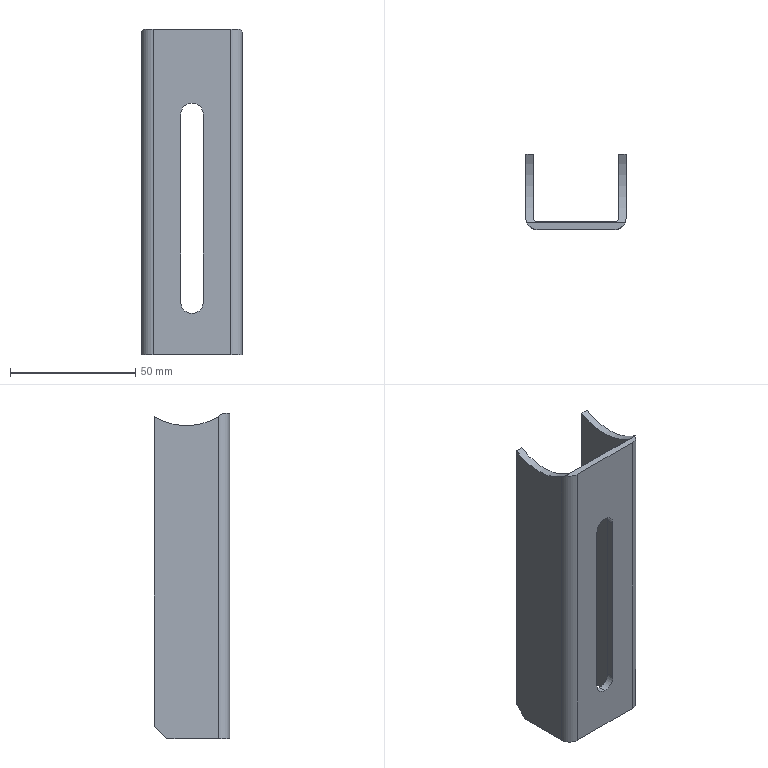Part | SolidWorks | features ICE 2, Chamfer 1, Extrusion 1 | 1 solid | 22 faces | box 40 x 30 x 130 mm | volume 32768 mm3 | plane 14 | cylinder 8 | commonest cylinder face diameters 9 x5 3 x2 48.3 x1
STEP:
#1=CARTESIAN_POINT('',(20.,-27.,16.5));
#2=VERTEX_POINT('',#1);
#3=CARTESIAN_POINT('',(24.5,-27.,21.));
#4=VERTEX_POINT('',#3);
#5=CARTESIAN_POINT('',(20.,-27.,21.));
#6=DIRECTION('',(0.,-1.,0.));
#7=DIRECTION('',(1.,0.,0.));
#8=AXIS2_PLACEMENT_3D('',#5,#6,#7);
#9=CIRCLE('',#8,4.5);
#10=EDGE_CURVE('',#2,#4,#9,.T.);
#11=ORIENTED_EDGE('',*,*,#10,.F.);
#12=CARTESIAN_POINT('',(20.,-30.,16.5));
#13=VERTEX_POINT('',#12);
#14=CARTESIAN_POINT('',(20.,100.,16.5));
#15=DIRECTION('',(0.,-1.,0.));
#16=VECTOR('',#15,1000.);
#17=LINE('',#14,#16);
#18=EDGE_CURVE('',#2,#13,#17,.T.);
#19=ORIENTED_EDGE('',*,*,#18,.T.);
#20=CARTESIAN_POINT('',(24.5,-30.,21.));
#21=VERTEX_POINT('',#20);
#22=CARTESIAN_POINT('',(20.,-30.,21.));
#23=DIRECTION('',(0.,-1.,0.));
#24=DIRECTION('',(0.,0.,-1.));
#25=AXIS2_PLACEMENT_3D('',#22,#23,#24);
#26=CIRCLE('',#25,4.5);
#27=EDGE_CURVE('',#13,#21,#26,.T.);
#28=ORIENTED_EDGE('',*,*,#27,.T.);
#29=CARTESIAN_POINT('',(24.5,100.,21.));
#30=DIRECTION('',(0.,-1.,0.));
#31=VECTOR('',#30,1000.);
#32=LINE('',#29,#31);
#33=EDGE_CURVE('',#4,#21,#32,.T.);
#34=ORIENTED_EDGE('',*,*,#33,.F.);
#35=EDGE_LOOP('',(#11,#19,#28,#34));
#36=FACE_OUTER_BOUND('',#35,.T.);
#37=CARTESIAN_POINT('',(20.,100.,21.));
#38=DIRECTION('',(0.,-1.,0.));
#39=DIRECTION('',(0.,0.,-1.));
#40=AXIS2_PLACEMENT_3D('',#37,#38,#39);
#41=CYLINDRICAL_SURFACE('',#40,4.5);
#42=ADVANCED_FACE('',(#36),#41,.F.);
#43=CARTESIAN_POINT('',(0.,0.,128.64));
#44=VERTEX_POINT('',#43);
#45=CARTESIAN_POINT('',(0.,0.,5.));
#46=VERTEX_POINT('',#45);
#47=CARTESIAN_POINT('',(0.,0.,130.));
#48=DIRECTION('',(0.,0.,-1.));
#49=VECTOR('',#48,1000.);
#50=LINE('',#47,#49);
#51=EDGE_CURVE('',#44,#46,#50,.T.);
#52=ORIENTED_EDGE('',*,*,#51,.F.);
#53=CARTESIAN_POINT('',(3.,0.,128.64));
#54=VERTEX_POINT('',#53);
#55=CARTESIAN_POINT('',(-90.,0.,128.64));
#56=DIRECTION('',(1.,0.,0.));
#57=VECTOR('',#56,1000.);
#58=LINE('',#55,#57);
#59=EDGE_CURVE('',#44,#54,#58,.T.);
#60=ORIENTED_EDGE('',*,*,#59,.T.);
#61=CARTESIAN_POINT('',(3.,0.,5.));
#62=VERTEX_POINT('',#61);
#63=CARTESIAN_POINT('',(3.,0.,130.));
#64=DIRECTION('',(0.,0.,-1.));
#65=VECTOR('',#64,1000.);
#66=LINE('',#63,#65);
#67=EDGE_CURVE('',#54,#62,#66,.T.);
#68=ORIENTED_EDGE('',*,*,#67,.T.);
#69=CARTESIAN_POINT('',(3.,0.,5.));
#70=DIRECTION('',(-1.,0.,0.));
#71=VECTOR('',#70,1000.);
#72=LINE('',#69,#71);
#73=EDGE_CURVE('',#62,#46,#72,.T.);
#74=ORIENTED_EDGE('',*,*,#73,.T.);
#75=EDGE_LOOP('',(#52,#60,#68,#74));
#76=FACE_OUTER_BOUND('',#75,.T.);
#77=CARTESIAN_POINT('',(3.,0.,130.));
#78=DIRECTION('',(0.,-1.,0.));
#79=DIRECTION('',(0.,0.,-1.));
#80=AXIS2_PLACEMENT_3D('',#77,#78,#79);
#81=PLANE('',#80);
#82=ADVANCED_FACE('',(#76),#81,.F.);
#83=CARTESIAN_POINT('',(0.,-25.5,128.64));
#84=VERTEX_POINT('',#83);
#85=CARTESIAN_POINT('',(0.,-25.5,0.));
#86=VERTEX_POINT('',#85);
#87=CARTESIAN_POINT('',(0.,-25.5,130.));
#88=DIRECTION('',(0.,0.,-1.));
#89=VECTOR('',#88,1000.);
#90=LINE('',#87,#89);
#91=EDGE_CURVE('',#84,#86,#90,.T.);
#92=ORIENTED_EDGE('',*,*,#91,.F.);
#93=CARTESIAN_POINT('',(0.,-12.75,149.15));
#94=DIRECTION('',(1.,0.,0.));
#95=DIRECTION('',(0.,1.,0.));
#96=AXIS2_PLACEMENT_3D('',#93,#94,#95);
#97=CIRCLE('',#96,24.15);
#98=EDGE_CURVE('',#84,#44,#97,.T.);
#99=ORIENTED_EDGE('',*,*,#98,.T.);
#100=ORIENTED_EDGE('',*,*,#51,.T.);
#101=CARTESIAN_POINT('',(0.,-5.,0.));
#102=VERTEX_POINT('',#101);
#103=CARTESIAN_POINT('',(0.,0.,5.));
#104=DIRECTION('',(0.,-0.7071,-0.7071));
#105=VECTOR('',#104,1000.);
#106=LINE('',#103,#105);
#107=EDGE_CURVE('',#46,#102,#106,.T.);
#108=ORIENTED_EDGE('',*,*,#107,.T.);
#109=CARTESIAN_POINT('',(0.,0.,0.));
#110=DIRECTION('',(0.,-1.,0.));
#111=VECTOR('',#110,1000.);
#112=LINE('',#109,#111);
#113=EDGE_CURVE('',#102,#86,#112,.T.);
#114=ORIENTED_EDGE('',*,*,#113,.T.);
#115=EDGE_LOOP('',(#92,#99,#100,#108,#114));
#116=FACE_OUTER_BOUND('',#115,.T.);
#117=CARTESIAN_POINT('',(0.,0.,130.));
#118=DIRECTION('',(1.,0.,0.));
#119=DIRECTION('',(0.,1.,0.));
#120=AXIS2_PLACEMENT_3D('',#117,#118,#119);
#121=PLANE('',#120);
#122=ADVANCED_FACE('',(#116),#121,.F.);
#123=CARTESIAN_POINT('',(0.4512,-27.464,130.));
#124=VERTEX_POINT('',#123);
#125=CARTESIAN_POINT('',(4.5,-30.,130.));
#126=VERTEX_POINT('',#125);
#127=CARTESIAN_POINT('',(4.5,-25.5,130.));
#128=DIRECTION('',(0.,0.,1.));
#129=DIRECTION('',(1.,0.,0.));
#130=AXIS2_PLACEMENT_3D('',#127,#128,#129);
#131=CIRCLE('',#130,4.5);
#132=EDGE_CURVE('',#124,#126,#131,.T.);
#133=ORIENTED_EDGE('',*,*,#132,.F.);
#134=CARTESIAN_POINT('',(0.4512,-27.464,130.));
#135=CARTESIAN_POINT('',(0.3031,-27.159,129.766));
#136=CARTESIAN_POINT('',(0.1919,-26.843,129.534));
#137=CARTESIAN_POINT('',(0.04037,-26.189,129.081));
#138=CARTESIAN_POINT('',(0.,-25.851,128.858));
#139=CARTESIAN_POINT('',(0.,-25.5,128.64));
#140=B_SPLINE_CURVE_WITH_KNOTS('',3,(#134,#135,#136,#137,#138,#139),.UNSPECIFIED.,.F.,.F.,(4,2,4),(0.,0.001216,0.002431),.UNSPECIFIED.);
#141=EDGE_CURVE('',#124,#84,#140,.T.);
#142=ORIENTED_EDGE('',*,*,#141,.T.);
#143=ORIENTED_EDGE('',*,*,#91,.T.);
#144=CARTESIAN_POINT('',(4.5,-30.,0.));
#145=VERTEX_POINT('',#144);
#146=CARTESIAN_POINT('',(4.5,-25.5,0.));
#147=DIRECTION('',(0.,0.,1.));
#148=DIRECTION('',(1.,0.,0.));
#149=AXIS2_PLACEMENT_3D('',#146,#147,#148);
#150=CIRCLE('',#149,4.5);
#151=EDGE_CURVE('',#86,#145,#150,.T.);
#152=ORIENTED_EDGE('',*,*,#151,.T.);
#153=CARTESIAN_POINT('',(4.5,-30.,130.));
#154=DIRECTION('',(0.,0.,-1.));
#155=VECTOR('',#154,1000.);
#156=LINE('',#153,#155);
#157=EDGE_CURVE('',#126,#145,#156,.T.);
#158=ORIENTED_EDGE('',*,*,#157,.F.);
#159=EDGE_LOOP('',(#133,#142,#143,#152,#158));
#160=FACE_OUTER_BOUND('',#159,.T.);
#161=CARTESIAN_POINT('',(4.5,-25.5,130.));
#162=DIRECTION('',(0.,0.,-1.));
#163=DIRECTION('',(-1.,0.,0.));
#164=AXIS2_PLACEMENT_3D('',#161,#162,#163);
#165=CYLINDRICAL_SURFACE('',#164,4.5);
#166=ADVANCED_FACE('',(#160),#165,.T.);
#167=CARTESIAN_POINT('',(15.5,-30.,96.));
#168=VERTEX_POINT('',#167);
#169=CARTESIAN_POINT('',(15.5,-30.,21.));
#170=VERTEX_POINT('',#169);
#171=CARTESIAN_POINT('',(15.5,-30.,96.));
#172=DIRECTION('',(0.,0.,-1.));
#173=VECTOR('',#172,1000.);
#174=LINE('',#171,#173);
#175=EDGE_CURVE('',#168,#170,#174,.T.);
#176=ORIENTED_EDGE('',*,*,#175,.F.);
#177=CARTESIAN_POINT('',(24.5,-30.,96.));
#178=VERTEX_POINT('',#177);
#179=CARTESIAN_POINT('',(20.,-30.,96.));
#180=DIRECTION('',(0.,-1.,0.));
#181=DIRECTION('',(0.,0.,-1.));
#182=AXIS2_PLACEMENT_3D('',#179,#180,#181);
#183=CIRCLE('',#182,4.5);
#184=EDGE_CURVE('',#178,#168,#183,.T.);
#185=ORIENTED_EDGE('',*,*,#184,.F.);
#186=CARTESIAN_POINT('',(24.5,-30.,96.));
#187=DIRECTION('',(0.,0.,1.));
#188=VECTOR('',#187,1000.);
#189=LINE('',#186,#188);
#190=EDGE_CURVE('',#21,#178,#189,.T.);
#191=ORIENTED_EDGE('',*,*,#190,.F.);
#192=ORIENTED_EDGE('',*,*,#27,.F.);
#193=CARTESIAN_POINT('',(20.,-30.,21.));
#194=DIRECTION('',(0.,-1.,0.));
#195=DIRECTION('',(0.,0.,-1.));
#196=AXIS2_PLACEMENT_3D('',#193,#194,#195);
#197=CIRCLE('',#196,4.5);
#198=EDGE_CURVE('',#170,#13,#197,.T.);
#199=ORIENTED_EDGE('',*,*,#198,.F.);
#200=EDGE_LOOP('',(#176,#185,#191,#192,#199));
#201=FACE_BOUND('',#200,.T.);
#202=CARTESIAN_POINT('',(35.5,-30.,0.));
#203=VERTEX_POINT('',#202);
#204=CARTESIAN_POINT('',(4.5,-30.,0.));
#205=DIRECTION('',(1.,0.,0.));
#206=VECTOR('',#205,1000.);
#207=LINE('',#204,#206);
#208=EDGE_CURVE('',#145,#203,#207,.T.);
#209=ORIENTED_EDGE('',*,*,#208,.T.);
#210=CARTESIAN_POINT('',(35.5,-30.,130.));
#211=VERTEX_POINT('',#210);
#212=CARTESIAN_POINT('',(35.5,-30.,130.));
#213=DIRECTION('',(0.,0.,-1.));
#214=VECTOR('',#213,1000.);
#215=LINE('',#212,#214);
#216=EDGE_CURVE('',#211,#203,#215,.T.);
#217=ORIENTED_EDGE('',*,*,#216,.F.);
#218=CARTESIAN_POINT('',(4.5,-30.,130.));
#219=DIRECTION('',(1.,0.,0.));
#220=VECTOR('',#219,1000.);
#221=LINE('',#218,#220);
#222=EDGE_CURVE('',#126,#211,#221,.T.);
#223=ORIENTED_EDGE('',*,*,#222,.F.);
#224=ORIENTED_EDGE('',*,*,#157,.T.);
#225=EDGE_LOOP('',(#209,#217,#223,#224));
#226=FACE_OUTER_BOUND('',#225,.T.);
#227=CARTESIAN_POINT('',(4.5,-30.,130.));
#228=DIRECTION('',(0.,1.,0.));
#229=DIRECTION('',(0.,0.,1.));
#230=AXIS2_PLACEMENT_3D('',#227,#228,#229);
#231=PLANE('',#230);
#232=ADVANCED_FACE('',(#201,#226),#231,.F.);
#233=CARTESIAN_POINT('',(40.,-25.5,128.64));
#234=VERTEX_POINT('',#233);
#235=CARTESIAN_POINT('',(40.,-25.5,0.));
#236=VERTEX_POINT('',#235);
#237=CARTESIAN_POINT('',(40.,-25.5,130.));
#238=DIRECTION('',(0.,0.,-1.));
#239=VECTOR('',#238,1000.);
#240=LINE('',#237,#239);
#241=EDGE_CURVE('',#234,#236,#240,.T.);
#242=ORIENTED_EDGE('',*,*,#241,.F.);
#243=CARTESIAN_POINT('',(39.549,-27.464,130.));
#244=VERTEX_POINT('',#243);
#245=CARTESIAN_POINT('',(40.,-25.5,128.64));
#246=CARTESIAN_POINT('',(40.,-25.851,128.858));
#247=CARTESIAN_POINT('',(39.96,-26.189,129.081));
#248=CARTESIAN_POINT('',(39.808,-26.843,129.534));
#249=CARTESIAN_POINT('',(39.697,-27.159,129.766));
#250=CARTESIAN_POINT('',(39.549,-27.464,130.));
#251=B_SPLINE_CURVE_WITH_KNOTS('',3,(#245,#246,#247,#248,#249,#250),.UNSPECIFIED.,.F.,.F.,(4,2,4),(0.,0.001216,0.002431),.UNSPECIFIED.);
#252=EDGE_CURVE('',#234,#244,#251,.T.);
#253=ORIENTED_EDGE('',*,*,#252,.T.);
#254=CARTESIAN_POINT('',(35.5,-25.5,130.));
#255=DIRECTION('',(0.,0.,1.));
#256=DIRECTION('',(1.,0.,0.));
#257=AXIS2_PLACEMENT_3D('',#254,#255,#256);
#258=CIRCLE('',#257,4.5);
#259=EDGE_CURVE('',#211,#244,#258,.T.);
#260=ORIENTED_EDGE('',*,*,#259,.F.);
#261=ORIENTED_EDGE('',*,*,#216,.T.);
#262=CARTESIAN_POINT('',(35.5,-25.5,0.));
#263=DIRECTION('',(0.,0.,1.));
#264=DIRECTION('',(1.,0.,0.));
#265=AXIS2_PLACEMENT_3D('',#262,#263,#264);
#266=CIRCLE('',#265,4.5);
#267=EDGE_CURVE('',#203,#236,#266,.T.);
#268=ORIENTED_EDGE('',*,*,#267,.T.);
#269=EDGE_LOOP('',(#242,#253,#260,#261,#268));
#270=FACE_OUTER_BOUND('',#269,.T.);
#271=CARTESIAN_POINT('',(35.5,-25.5,130.));
#272=DIRECTION('',(0.,0.,-1.));
#273=DIRECTION('',(-1.,0.,0.));
#274=AXIS2_PLACEMENT_3D('',#271,#272,#273);
#275=CYLINDRICAL_SURFACE('',#274,4.5);
#276=ADVANCED_FACE('',(#270),#275,.T.);
#277=CARTESIAN_POINT('',(40.,0.,128.64));
#278=VERTEX_POINT('',#277);
#279=CARTESIAN_POINT('',(40.,0.,5.));
#280=VERTEX_POINT('',#279);
#281=CARTESIAN_POINT('',(40.,0.,130.));
#282=DIRECTION('',(0.,0.,-1.));
#283=VECTOR('',#282,1000.);
#284=LINE('',#281,#283);
#285=EDGE_CURVE('',#278,#280,#284,.T.);
#286=ORIENTED_EDGE('',*,*,#285,.F.);
#287=CARTESIAN_POINT('',(40.,-12.75,149.15));
#288=DIRECTION('',(1.,0.,0.));
#289=DIRECTION('',(0.,1.,0.));
#290=AXIS2_PLACEMENT_3D('',#287,#288,#289);
#291=CIRCLE('',#290,24.15);
#292=EDGE_CURVE('',#234,#278,#291,.T.);
#293=ORIENTED_EDGE('',*,*,#292,.F.);
#294=ORIENTED_EDGE('',*,*,#241,.T.);
#295=CARTESIAN_POINT('',(40.,-5.,0.));
#296=VERTEX_POINT('',#295);
#297=CARTESIAN_POINT('',(40.,-25.5,0.));
#298=DIRECTION('',(0.,1.,0.));
#299=VECTOR('',#298,1000.);
#300=LINE('',#297,#299);
#301=EDGE_CURVE('',#236,#296,#300,.T.);
#302=ORIENTED_EDGE('',*,*,#301,.T.);
#303=CARTESIAN_POINT('',(40.,0.,5.));
#304=DIRECTION('',(0.,0.7071,0.7071));
#305=VECTOR('',#304,1000.);
#306=LINE('',#303,#305);
#307=EDGE_CURVE('',#296,#280,#306,.T.);
#308=ORIENTED_EDGE('',*,*,#307,.T.);
#309=EDGE_LOOP('',(#286,#293,#294,#302,#308));
#310=FACE_OUTER_BOUND('',#309,.T.);
#311=CARTESIAN_POINT('',(40.,-25.5,130.));
#312=DIRECTION('',(-1.,0.,0.));
#313=DIRECTION('',(0.,-1.,0.));
#314=AXIS2_PLACEMENT_3D('',#311,#312,#313);
#315=PLANE('',#314);
#316=ADVANCED_FACE('',(#310),#315,.F.);
#317=CARTESIAN_POINT('',(37.,0.,128.64));
#318=VERTEX_POINT('',#317);
#319=CARTESIAN_POINT('',(37.,0.,5.));
#320=VERTEX_POINT('',#319);
#321=CARTESIAN_POINT('',(37.,0.,130.));
#322=DIRECTION('',(0.,0.,-1.));
#323=VECTOR('',#322,1000.);
#324=LINE('',#321,#323);
#325=EDGE_CURVE('',#318,#320,#324,.T.);
#326=ORIENTED_EDGE('',*,*,#325,.F.);
#327=CARTESIAN_POINT('',(-90.,0.,128.64));
#328=DIRECTION('',(1.,0.,0.));
#329=VECTOR('',#328,1000.);
#330=LINE('',#327,#329);
#331=EDGE_CURVE('',#318,#278,#330,.T.);
#332=ORIENTED_EDGE('',*,*,#331,.T.);
#333=ORIENTED_EDGE('',*,*,#285,.T.);
#334=CARTESIAN_POINT('',(37.,0.,5.));
#335=DIRECTION('',(-1.,0.,0.));
#336=VECTOR('',#335,1000.);
#337=LINE('',#334,#336);
#338=EDGE_CURVE('',#280,#320,#337,.T.);
#339=ORIENTED_EDGE('',*,*,#338,.T.);
#340=EDGE_LOOP('',(#326,#332,#333,#339));
#341=FACE_OUTER_BOUND('',#340,.T.);
#342=CARTESIAN_POINT('',(37.,0.,130.));
#343=DIRECTION('',(0.,-1.,0.));
#344=DIRECTION('',(0.,0.,-1.));
#345=AXIS2_PLACEMENT_3D('',#342,#343,#344);
#346=PLANE('',#345);
#347=ADVANCED_FACE('',(#341),#346,.F.);
#348=CARTESIAN_POINT('',(37.,-25.5,128.64));
#349=VERTEX_POINT('',#348);
#350=CARTESIAN_POINT('',(37.,-25.5,0.));
#351=VERTEX_POINT('',#350);
#352=CARTESIAN_POINT('',(37.,-25.5,130.));
#353=DIRECTION('',(0.,0.,-1.));
#354=VECTOR('',#353,1000.);
#355=LINE('',#352,#354);
#356=EDGE_CURVE('',#349,#351,#355,.T.);
#357=ORIENTED_EDGE('',*,*,#356,.F.);
#358=CARTESIAN_POINT('',(37.,-12.75,149.15));
#359=DIRECTION('',(1.,0.,0.));
#360=DIRECTION('',(0.,1.,0.));
#361=AXIS2_PLACEMENT_3D('',#358,#359,#360);
#362=CIRCLE('',#361,24.15);
#363=EDGE_CURVE('',#349,#318,#362,.T.);
#364=ORIENTED_EDGE('',*,*,#363,.T.);
#365=ORIENTED_EDGE('',*,*,#325,.T.);
#366=CARTESIAN_POINT('',(37.,-5.,0.));
#367=VERTEX_POINT('',#366);
#368=CARTESIAN_POINT('',(37.,0.,5.));
#369=DIRECTION('',(0.,-0.7071,-0.7071));
#370=VECTOR('',#369,1000.);
#371=LINE('',#368,#370);
#372=EDGE_CURVE('',#320,#367,#371,.T.);
#373=ORIENTED_EDGE('',*,*,#372,.T.);
#374=CARTESIAN_POINT('',(37.,-25.5,0.));
#375=DIRECTION('',(0.,-1.,0.));
#376=VECTOR('',#375,1000.);
#377=LINE('',#374,#376);
#378=EDGE_CURVE('',#367,#351,#377,.T.);
#379=ORIENTED_EDGE('',*,*,#378,.T.);
#380=EDGE_LOOP('',(#357,#364,#365,#373,#379));
#381=FACE_OUTER_BOUND('',#380,.T.);
#382=CARTESIAN_POINT('',(37.,-25.5,130.));
#383=DIRECTION('',(1.,0.,0.));
#384=DIRECTION('',(0.,1.,0.));
#385=AXIS2_PLACEMENT_3D('',#382,#383,#384);
#386=PLANE('',#385);
#387=ADVANCED_FACE('',(#381),#386,.F.);
#388=CARTESIAN_POINT('',(35.5,-27.,129.652));
#389=VERTEX_POINT('',#388);
#390=CARTESIAN_POINT('',(35.5,-27.,0.));
#391=VERTEX_POINT('',#390);
#392=CARTESIAN_POINT('',(35.5,-27.,130.));
#393=DIRECTION('',(0.,0.,-1.));
#394=VECTOR('',#393,1000.);
#395=LINE('',#392,#394);
#396=EDGE_CURVE('',#389,#391,#395,.T.);
#397=ORIENTED_EDGE('',*,*,#396,.F.);
#398=CARTESIAN_POINT('',(35.5,-27.,129.652));
#399=CARTESIAN_POINT('',(35.61,-27.,129.652));
#400=CARTESIAN_POINT('',(35.716,-26.988,129.644));
#401=CARTESIAN_POINT('',(35.925,-26.942,129.61));
#402=CARTESIAN_POINT('',(36.027,-26.908,129.585));
#403=CARTESIAN_POINT('',(36.216,-26.822,129.524));
#404=CARTESIAN_POINT('',(36.305,-26.77,129.486));
#405=CARTESIAN_POINT('',(36.466,-26.652,129.402));
#406=CARTESIAN_POINT('',(36.539,-26.586,129.356));
#407=CARTESIAN_POINT('',(36.736,-26.372,129.208));
#408=CARTESIAN_POINT('',(36.834,-26.21,129.098));
#409=CARTESIAN_POINT('',(36.967,-25.864,128.87));
#410=CARTESIAN_POINT('',(37.,-25.685,128.755));
#411=CARTESIAN_POINT('',(37.,-25.5,128.64));
#412=B_SPLINE_CURVE_WITH_KNOTS('',3,(#398,#399,#400,#401,#402,#403,#404,#405,#406,#407,#408,#409,#410,#411),.UNSPECIFIED.,.F.,.F.,(4,2,2,2,2,2,4),(0.,0.0003234,0.0006469,0.0009703,0.001294,0.001941,0.002588),.UNSPECIFIED.);
#413=EDGE_CURVE('',#389,#349,#412,.T.);
#414=ORIENTED_EDGE('',*,*,#413,.T.);
#415=ORIENTED_EDGE('',*,*,#356,.T.);
#416=CARTESIAN_POINT('',(35.5,-25.5,0.));
#417=DIRECTION('',(0.,0.,-1.));
#418=DIRECTION('',(1.,0.,0.));
#419=AXIS2_PLACEMENT_3D('',#416,#417,#418);
#420=CIRCLE('',#419,1.5);
#421=EDGE_CURVE('',#351,#391,#420,.T.);
#422=ORIENTED_EDGE('',*,*,#421,.T.);
#423=EDGE_LOOP('',(#397,#414,#415,#422));
#424=FACE_OUTER_BOUND('',#423,.T.);
#425=CARTESIAN_POINT('',(35.5,-25.5,130.));
#426=DIRECTION('',(0.,0.,-1.));
#427=DIRECTION('',(-1.,0.,0.));
#428=AXIS2_PLACEMENT_3D('',#425,#426,#427);
#429=CYLINDRICAL_SURFACE('',#428,1.5);
#430=ADVANCED_FACE('',(#424),#429,.F.);
#431=CARTESIAN_POINT('',(24.5,-27.,96.));
#432=VERTEX_POINT('',#431);
#433=CARTESIAN_POINT('',(24.5,-27.,130.));
#434=DIRECTION('',(0.,0.,1.));
#435=VECTOR('',#434,1000.);
#436=LINE('',#433,#435);
#437=EDGE_CURVE('',#4,#432,#436,.T.);
#438=ORIENTED_EDGE('',*,*,#437,.T.);
#439=CARTESIAN_POINT('',(15.5,-27.,96.));
#440=VERTEX_POINT('',#439);
#441=CARTESIAN_POINT('',(20.,-27.,96.));
#442=DIRECTION('',(0.,-1.,0.));
#443=DIRECTION('',(1.,0.,0.));
#444=AXIS2_PLACEMENT_3D('',#441,#442,#443);
#445=CIRCLE('',#444,4.5);
#446=EDGE_CURVE('',#432,#440,#445,.T.);
#447=ORIENTED_EDGE('',*,*,#446,.T.);
#448=CARTESIAN_POINT('',(15.5,-27.,21.));
#449=VERTEX_POINT('',#448);
#450=CARTESIAN_POINT('',(15.5,-27.,130.));
#451=DIRECTION('',(0.,0.,-1.));
#452=VECTOR('',#451,1000.);
#453=LINE('',#450,#452);
#454=EDGE_CURVE('',#440,#449,#453,.T.);
#455=ORIENTED_EDGE('',*,*,#454,.T.);
#456=CARTESIAN_POINT('',(20.,-27.,21.));
#457=DIRECTION('',(0.,-1.,0.));
#458=DIRECTION('',(1.,0.,0.));
#459=AXIS2_PLACEMENT_3D('',#456,#457,#458);
#460=CIRCLE('',#459,4.5);
#461=EDGE_CURVE('',#449,#2,#460,.T.);
#462=ORIENTED_EDGE('',*,*,#461,.T.);
#463=ORIENTED_EDGE('',*,*,#10,.T.);
#464=EDGE_LOOP('',(#438,#447,#455,#462,#463));
#465=FACE_BOUND('',#464,.T.);
#466=CARTESIAN_POINT('',(4.5,-27.,129.652));
#467=VERTEX_POINT('',#466);
#468=CARTESIAN_POINT('',(4.5,-27.,0.));
#469=VERTEX_POINT('',#468);
#470=CARTESIAN_POINT('',(4.5,-27.,130.));
#471=DIRECTION('',(0.,0.,-1.));
#472=VECTOR('',#471,1000.);
#473=LINE('',#470,#472);
#474=EDGE_CURVE('',#467,#469,#473,.T.);
#475=ORIENTED_EDGE('',*,*,#474,.F.);
#476=CARTESIAN_POINT('',(-90.,-27.,129.652));
#477=DIRECTION('',(1.,0.,0.));
#478=VECTOR('',#477,1000.);
#479=LINE('',#476,#478);
#480=EDGE_CURVE('',#467,#389,#479,.T.);
#481=ORIENTED_EDGE('',*,*,#480,.T.);
#482=ORIENTED_EDGE('',*,*,#396,.T.);
#483=CARTESIAN_POINT('',(4.5,-27.,0.));
#484=DIRECTION('',(-1.,0.,0.));
#485=VECTOR('',#484,1000.);
#486=LINE('',#483,#485);
#487=EDGE_CURVE('',#391,#469,#486,.T.);
#488=ORIENTED_EDGE('',*,*,#487,.T.);
#489=EDGE_LOOP('',(#475,#481,#482,#488));
#490=FACE_OUTER_BOUND('',#489,.T.);
#491=CARTESIAN_POINT('',(4.5,-27.,130.));
#492=DIRECTION('',(0.,-1.,0.));
#493=DIRECTION('',(1.,0.,0.));
#494=AXIS2_PLACEMENT_3D('',#491,#492,#493);
#495=PLANE('',#494);
#496=ADVANCED_FACE('',(#465,#490),#495,.F.);
#497=CARTESIAN_POINT('',(3.,-25.5,128.64));
#498=VERTEX_POINT('',#497);
#499=CARTESIAN_POINT('',(3.,-25.5,0.));
#500=VERTEX_POINT('',#499);
#501=CARTESIAN_POINT('',(3.,-25.5,130.));
#502=DIRECTION('',(0.,0.,-1.));
#503=VECTOR('',#502,1000.);
#504=LINE('',#501,#503);
#505=EDGE_CURVE('',#498,#500,#504,.T.);
#506=ORIENTED_EDGE('',*,*,#505,.F.);
#507=CARTESIAN_POINT('',(3.,-25.5,128.64));
#508=CARTESIAN_POINT('',(3.,-25.686,128.755));
#509=CARTESIAN_POINT('',(3.033,-25.864,128.87));
#510=CARTESIAN_POINT('',(3.132,-26.123,129.04));
#511=CARTESIAN_POINT('',(3.174,-26.207,129.097));
#512=CARTESIAN_POINT('',(3.272,-26.367,129.205));
#513=CARTESIAN_POINT('',(3.329,-26.442,129.256));
#514=CARTESIAN_POINT('',(3.458,-26.584,129.355));
#515=CARTESIAN_POINT('',(3.533,-26.651,129.402));
#516=CARTESIAN_POINT('',(3.694,-26.769,129.485));
#517=CARTESIAN_POINT('',(3.781,-26.821,129.523));
#518=CARTESIAN_POINT('',(3.972,-26.908,129.585));
#519=CARTESIAN_POINT('',(4.073,-26.942,129.61));
#520=CARTESIAN_POINT('',(4.281,-26.988,129.643));
#521=CARTESIAN_POINT('',(4.39,-27.,129.652));
#522=CARTESIAN_POINT('',(4.5,-27.,129.652));
#523=B_SPLINE_CURVE_WITH_KNOTS('',3,(#507,#508,#509,#510,#511,#512,#513,#514,#515,#516,#517,#518,#519,#520,#521,#522),.UNSPECIFIED.,.F.,.F.,(4,2,2,2,2,2,2,4),(0.,0.0006447,0.000967,0.001289,0.001612,0.001934,0.002256,0.002579),.UNSPECIFIED.);
#524=EDGE_CURVE('',#498,#467,#523,.T.);
#525=ORIENTED_EDGE('',*,*,#524,.T.);
#526=ORIENTED_EDGE('',*,*,#474,.T.);
#527=CARTESIAN_POINT('',(4.5,-25.5,0.));
#528=DIRECTION('',(0.,0.,-1.));
#529=DIRECTION('',(1.,0.,0.));
#530=AXIS2_PLACEMENT_3D('',#527,#528,#529);
#531=CIRCLE('',#530,1.5);
#532=EDGE_CURVE('',#469,#500,#531,.T.);
#533=ORIENTED_EDGE('',*,*,#532,.T.);
#534=EDGE_LOOP('',(#506,#525,#526,#533));
#535=FACE_OUTER_BOUND('',#534,.T.);
#536=CARTESIAN_POINT('',(4.5,-25.5,130.));
#537=DIRECTION('',(0.,0.,-1.));
#538=DIRECTION('',(-1.,0.,0.));
#539=AXIS2_PLACEMENT_3D('',#536,#537,#538);
#540=CYLINDRICAL_SURFACE('',#539,1.5);
#541=ADVANCED_FACE('',(#535),#540,.F.);
#542=ORIENTED_EDGE('',*,*,#67,.F.);
#543=CARTESIAN_POINT('',(3.,-12.75,149.15));
#544=DIRECTION('',(-1.,0.,0.));
#545=DIRECTION('',(0.,-1.,0.));
#546=AXIS2_PLACEMENT_3D('',#543,#544,#545);
#547=CIRCLE('',#546,24.15);
#548=EDGE_CURVE('',#54,#498,#547,.T.);
#549=ORIENTED_EDGE('',*,*,#548,.T.);
#550=ORIENTED_EDGE('',*,*,#505,.T.);
#551=CARTESIAN_POINT('',(3.,-5.,0.));
#552=VERTEX_POINT('',#551);
#553=CARTESIAN_POINT('',(3.,0.,0.));
#554=DIRECTION('',(0.,1.,0.));
#555=VECTOR('',#554,1000.);
#556=LINE('',#553,#555);
#557=EDGE_CURVE('',#500,#552,#556,.T.);
#558=ORIENTED_EDGE('',*,*,#557,.T.);
#559=CARTESIAN_POINT('',(3.,0.,5.));
#560=DIRECTION('',(0.,0.7071,0.7071));
#561=VECTOR('',#560,1000.);
#562=LINE('',#559,#561);
#563=EDGE_CURVE('',#552,#62,#562,.T.);
#564=ORIENTED_EDGE('',*,*,#563,.T.);
#565=EDGE_LOOP('',(#542,#549,#550,#558,#564));
#566=FACE_OUTER_BOUND('',#565,.T.);
#567=CARTESIAN_POINT('',(3.,0.,130.));
#568=DIRECTION('',(-1.,0.,0.));
#569=DIRECTION('',(0.,-1.,0.));
#570=AXIS2_PLACEMENT_3D('',#567,#568,#569);
#571=PLANE('',#570);
#572=ADVANCED_FACE('',(#566),#571,.F.);
#573=CARTESIAN_POINT('',(-90.,-27.464,130.));
#574=DIRECTION('',(1.,0.,0.));
#575=VECTOR('',#574,1000.);
#576=LINE('',#573,#575);
#577=EDGE_CURVE('',#124,#244,#576,.T.);
#578=ORIENTED_EDGE('',*,*,#577,.F.);
#579=ORIENTED_EDGE('',*,*,#132,.T.);
#580=ORIENTED_EDGE('',*,*,#222,.T.);
#581=ORIENTED_EDGE('',*,*,#259,.T.);
#582=EDGE_LOOP('',(#578,#579,#580,#581));
#583=FACE_OUTER_BOUND('',#582,.T.);
#584=CARTESIAN_POINT('',(4.5,-25.5,130.));
#585=DIRECTION('',(0.,0.,1.));
#586=DIRECTION('',(1.,0.,0.));
#587=AXIS2_PLACEMENT_3D('',#584,#585,#586);
#588=PLANE('',#587);
#589=ADVANCED_FACE('',(#583),#588,.T.);
#590=ORIENTED_EDGE('',*,*,#113,.F.);
#591=CARTESIAN_POINT('',(4.5,-5.,0.));
#592=DIRECTION('',(1.,0.,0.));
#593=VECTOR('',#592,1000.);
#594=LINE('',#591,#593);
#595=EDGE_CURVE('',#102,#552,#594,.T.);
#596=ORIENTED_EDGE('',*,*,#595,.T.);
#597=ORIENTED_EDGE('',*,*,#557,.F.);
#598=ORIENTED_EDGE('',*,*,#532,.F.);
#599=ORIENTED_EDGE('',*,*,#487,.F.);
#600=ORIENTED_EDGE('',*,*,#421,.F.);
#601=ORIENTED_EDGE('',*,*,#378,.F.);
#602=CARTESIAN_POINT('',(4.5,-5.,0.));
#603=DIRECTION('',(1.,0.,0.));
#604=VECTOR('',#603,1000.);
#605=LINE('',#602,#604);
#606=EDGE_CURVE('',#367,#296,#605,.T.);
#607=ORIENTED_EDGE('',*,*,#606,.T.);
#608=ORIENTED_EDGE('',*,*,#301,.F.);
#609=ORIENTED_EDGE('',*,*,#267,.F.);
#610=ORIENTED_EDGE('',*,*,#208,.F.);
#611=ORIENTED_EDGE('',*,*,#151,.F.);
#612=EDGE_LOOP('',(#590,#596,#597,#598,#599,#600,#601,#607,#608,#609,#610,#611));
#613=FACE_OUTER_BOUND('',#612,.T.);
#614=CARTESIAN_POINT('',(4.5,-25.5,0.));
#615=DIRECTION('',(0.,0.,1.));
#616=DIRECTION('',(1.,0.,0.));
#617=AXIS2_PLACEMENT_3D('',#614,#615,#616);
#618=PLANE('',#617);
#619=ADVANCED_FACE('',(#613),#618,.F.);
#620=ORIENTED_EDGE('',*,*,#563,.F.);
#621=ORIENTED_EDGE('',*,*,#595,.F.);
#622=ORIENTED_EDGE('',*,*,#107,.F.);
#623=ORIENTED_EDGE('',*,*,#73,.F.);
#624=EDGE_LOOP('',(#620,#621,#622,#623));
#625=FACE_OUTER_BOUND('',#624,.T.);
#626=CARTESIAN_POINT('',(3.,0.,5.));
#627=DIRECTION('',(0.,-0.7071,0.7071));
#628=DIRECTION('',(-1.,0.,0.));
#629=AXIS2_PLACEMENT_3D('',#626,#627,#628);
#630=PLANE('',#629);
#631=ADVANCED_FACE('',(#625),#630,.F.);
#632=ORIENTED_EDGE('',*,*,#307,.F.);
#633=ORIENTED_EDGE('',*,*,#606,.F.);
#634=ORIENTED_EDGE('',*,*,#372,.F.);
#635=ORIENTED_EDGE('',*,*,#338,.F.);
#636=EDGE_LOOP('',(#632,#633,#634,#635));
#637=FACE_OUTER_BOUND('',#636,.T.);
#638=CARTESIAN_POINT('',(37.,0.,5.));
#639=DIRECTION('',(0.,-0.7071,0.7071));
#640=DIRECTION('',(-1.,0.,0.));
#641=AXIS2_PLACEMENT_3D('',#638,#639,#640);
#642=PLANE('',#641);
#643=ADVANCED_FACE('',(#637),#642,.F.);
#644=ORIENTED_EDGE('',*,*,#363,.F.);
#645=ORIENTED_EDGE('',*,*,#413,.F.);
#646=ORIENTED_EDGE('',*,*,#480,.F.);
#647=ORIENTED_EDGE('',*,*,#524,.F.);
#648=ORIENTED_EDGE('',*,*,#548,.F.);
#649=ORIENTED_EDGE('',*,*,#59,.F.);
#650=ORIENTED_EDGE('',*,*,#98,.F.);
#651=ORIENTED_EDGE('',*,*,#141,.F.);
#652=ORIENTED_EDGE('',*,*,#577,.T.);
#653=ORIENTED_EDGE('',*,*,#252,.F.);
#654=ORIENTED_EDGE('',*,*,#292,.T.);
#655=ORIENTED_EDGE('',*,*,#331,.F.);
#656=EDGE_LOOP('',(#644,#645,#646,#647,#648,#649,#650,#651,#652,#653,#654,#655));
#657=FACE_OUTER_BOUND('',#656,.T.);
#658=CARTESIAN_POINT('',(-90.,-12.75,149.15));
#659=DIRECTION('',(1.,0.,0.));
#660=DIRECTION('',(0.,1.,0.));
#661=AXIS2_PLACEMENT_3D('',#658,#659,#660);
#662=CYLINDRICAL_SURFACE('',#661,24.15);
#663=ADVANCED_FACE('',(#657),#662,.F.);
#664=CARTESIAN_POINT('',(24.5,100.,96.));
#665=DIRECTION('',(0.,-1.,0.));
#666=VECTOR('',#665,1000.);
#667=LINE('',#664,#666);
#668=EDGE_CURVE('',#432,#178,#667,.T.);
#669=ORIENTED_EDGE('',*,*,#668,.T.);
#670=ORIENTED_EDGE('',*,*,#184,.T.);
#671=CARTESIAN_POINT('',(15.5,100.,96.));
#672=DIRECTION('',(0.,-1.,0.));
#673=VECTOR('',#672,1000.);
#674=LINE('',#671,#673);
#675=EDGE_CURVE('',#440,#168,#674,.T.);
#676=ORIENTED_EDGE('',*,*,#675,.F.);
#677=ORIENTED_EDGE('',*,*,#446,.F.);
#678=EDGE_LOOP('',(#669,#670,#676,#677));
#679=FACE_OUTER_BOUND('',#678,.T.);
#680=CARTESIAN_POINT('',(20.,100.,96.));
#681=DIRECTION('',(0.,-1.,0.));
#682=DIRECTION('',(0.,0.,-1.));
#683=AXIS2_PLACEMENT_3D('',#680,#681,#682);
#684=CYLINDRICAL_SURFACE('',#683,4.5);
#685=ADVANCED_FACE('',(#679),#684,.F.);
#686=ORIENTED_EDGE('',*,*,#33,.T.);
#687=ORIENTED_EDGE('',*,*,#190,.T.);
#688=ORIENTED_EDGE('',*,*,#668,.F.);
#689=ORIENTED_EDGE('',*,*,#437,.F.);
#690=EDGE_LOOP('',(#686,#687,#688,#689));
#691=FACE_OUTER_BOUND('',#690,.T.);
#692=CARTESIAN_POINT('',(24.5,100.,96.));
#693=DIRECTION('',(1.,0.,0.));
#694=DIRECTION('',(0.,0.,-1.));
#695=AXIS2_PLACEMENT_3D('',#692,#693,#694);
#696=PLANE('',#695);
#697=ADVANCED_FACE('',(#691),#696,.F.);
#698=ORIENTED_EDGE('',*,*,#18,.F.);
#699=ORIENTED_EDGE('',*,*,#461,.F.);
#700=CARTESIAN_POINT('',(15.5,100.,21.));
#701=DIRECTION('',(0.,-1.,0.));
#702=VECTOR('',#701,1000.);
#703=LINE('',#700,#702);
#704=EDGE_CURVE('',#449,#170,#703,.T.);
#705=ORIENTED_EDGE('',*,*,#704,.T.);
#706=ORIENTED_EDGE('',*,*,#198,.T.);
#707=EDGE_LOOP('',(#698,#699,#705,#706));
#708=FACE_OUTER_BOUND('',#707,.T.);
#709=CARTESIAN_POINT('',(20.,100.,21.));
#710=DIRECTION('',(0.,-1.,0.));
#711=DIRECTION('',(0.,0.,-1.));
#712=AXIS2_PLACEMENT_3D('',#709,#710,#711);
#713=CYLINDRICAL_SURFACE('',#712,4.5);
#714=ADVANCED_FACE('',(#708),#713,.F.);
#715=ORIENTED_EDGE('',*,*,#675,.T.);
#716=ORIENTED_EDGE('',*,*,#175,.T.);
#717=ORIENTED_EDGE('',*,*,#704,.F.);
#718=ORIENTED_EDGE('',*,*,#454,.F.);
#719=EDGE_LOOP('',(#715,#716,#717,#718));
#720=FACE_OUTER_BOUND('',#719,.T.);
#721=CARTESIAN_POINT('',(15.5,100.,96.));
#722=DIRECTION('',(-1.,0.,0.));
#723=DIRECTION('',(0.,0.,1.));
#724=AXIS2_PLACEMENT_3D('',#721,#722,#723);
#725=PLANE('',#724);
#726=ADVANCED_FACE('',(#720),#725,.F.);
#727=CLOSED_SHELL('',(#42,#82,#122,#166,#232,#276,#316,#347,#387,#430,#496,#541,#572,#589,#619,#631,#643,#663,#685,#697,#714,#726));
#728=MANIFOLD_SOLID_BREP('',#727);
#729=CARTESIAN_POINT('',(0.,0.,0.));
#730=DIRECTION('',(0.,0.,1.));
#731=DIRECTION('',(1.,0.,0.));
#732=AXIS2_PLACEMENT_3D('',#729,#730,#731);
#733=(LENGTH_UNIT()NAMED_UNIT(*)SI_UNIT(.MILLI.,.METRE.));
#734=UNCERTAINTY_MEASURE_WITH_UNIT(LENGTH_MEASURE(0.00001),#733,'','');
#735=(NAMED_UNIT(*)PLANE_ANGLE_UNIT()SI_UNIT($,.RADIAN.));
#736=(NAMED_UNIT(*)SI_UNIT($,.STERADIAN.)SOLID_ANGLE_UNIT());
#737=(GEOMETRIC_REPRESENTATION_CONTEXT(3)GLOBAL_UNCERTAINTY_ASSIGNED_CONTEXT((#734))GLOBAL_UNIT_ASSIGNED_CONTEXT((#733,#735,#736))REPRESENTATION_CONTEXT('',''));
#738=ADVANCED_BREP_SHAPE_REPRESENTATION('',(#728,#732),#737);